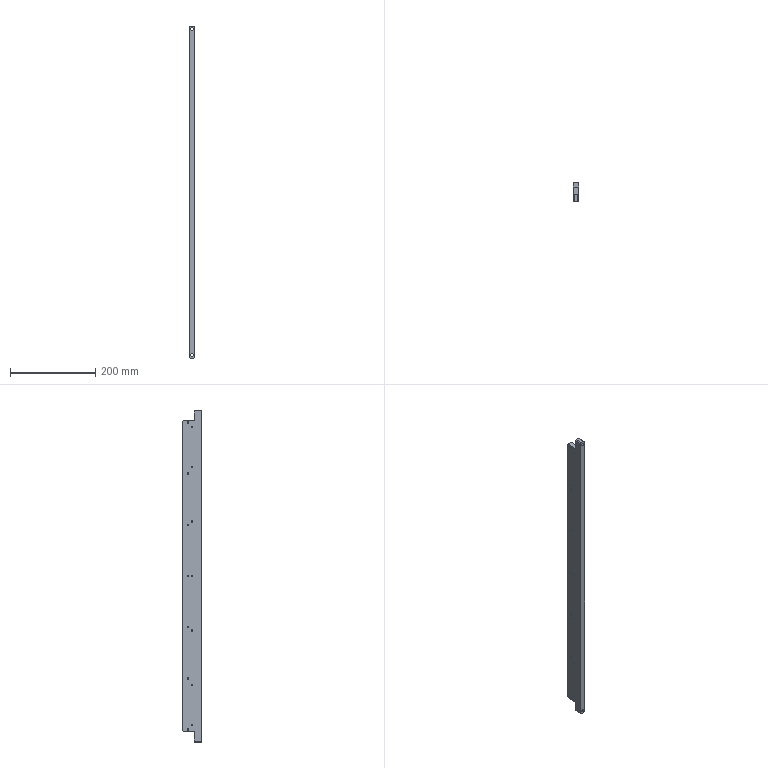Part | NX | features BREP 1 | 1 solid | 64 faces | box 12 x 45 x 778 mm | volume 399917 mm3 | cylinder 40 | plane 16 | cone 8 | commonest cylinder face diameters 3.3 x36 7 x4